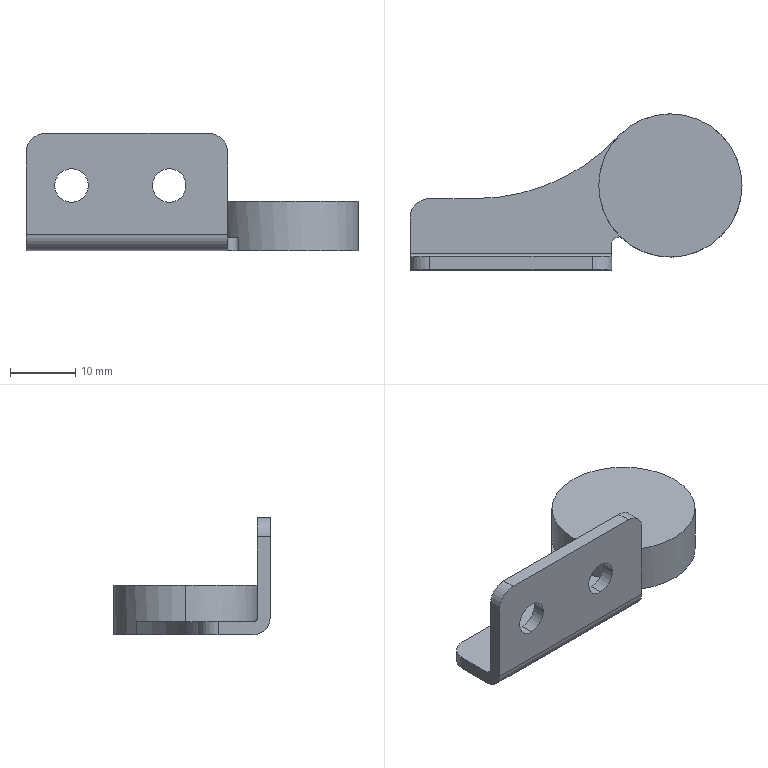Part | SolidWorks | features BaseBody 1 | 1 solid | 42 faces | box 51 x 24 x 18 mm | volume 4464 mm3 | cylinder 25 | plane 17 | commonest cylinder face diameters 0.528 x8 5.153 x4 6 x3 10 x2 10.02 x2 22 x2
STEP:
#1=CARTESIAN_POINT('',(-8.035,10.178,3.237));
#2=VERTEX_POINT('',#1);
#3=CARTESIAN_POINT('',(-11.,2.666,3.237));
#4=VERTEX_POINT('',#3);
#5=CARTESIAN_POINT('',(0.,2.666,3.237));
#6=DIRECTION('',(0.,0.,1.));
#7=DIRECTION('',(1.,0.,0.));
#8=AXIS2_PLACEMENT_3D('',#5,#6,#7);
#9=CIRCLE('',#8,11.);
#10=EDGE_CURVE('',#2,#4,#9,.T.);
#11=ORIENTED_EDGE('',*,*,#10,.T.);
#12=CARTESIAN_POINT('',(-11.,2.666,8.837));
#13=VERTEX_POINT('',#12);
#14=CARTESIAN_POINT('',(-11.,2.666,1.237));
#15=DIRECTION('',(0.,0.,1.));
#16=VECTOR('',#15,1000.);
#17=LINE('',#14,#16);
#18=EDGE_CURVE('',#4,#13,#17,.T.);
#19=ORIENTED_EDGE('',*,*,#18,.T.);
#20=CARTESIAN_POINT('',(11.,2.666,8.837));
#21=VERTEX_POINT('',#20);
#22=CARTESIAN_POINT('',(0.,2.666,8.837));
#23=DIRECTION('',(0.,0.,-1.));
#24=DIRECTION('',(1.,0.,0.));
#25=AXIS2_PLACEMENT_3D('',#22,#23,#24);
#26=CIRCLE('',#25,11.);
#27=EDGE_CURVE('',#13,#21,#26,.T.);
#28=ORIENTED_EDGE('',*,*,#27,.T.);
#29=CARTESIAN_POINT('',(11.,2.666,1.237));
#30=VERTEX_POINT('',#29);
#31=CARTESIAN_POINT('',(11.,2.666,1.237));
#32=DIRECTION('',(0.,0.,1.));
#33=VECTOR('',#32,1000.);
#34=LINE('',#31,#33);
#35=EDGE_CURVE('',#30,#21,#34,.T.);
#36=ORIENTED_EDGE('',*,*,#35,.F.);
#37=CARTESIAN_POINT('',(-8.035,10.178,1.237));
#38=VERTEX_POINT('',#37);
#39=CARTESIAN_POINT('',(0.,2.666,1.237));
#40=DIRECTION('',(0.,0.,-1.));
#41=DIRECTION('',(1.,0.,0.));
#42=AXIS2_PLACEMENT_3D('',#39,#40,#41);
#43=CIRCLE('',#42,11.);
#44=EDGE_CURVE('',#38,#30,#43,.T.);
#45=ORIENTED_EDGE('',*,*,#44,.F.);
#46=CARTESIAN_POINT('',(-8.035,10.178,1.237));
#47=DIRECTION('',(0.,0.,1.));
#48=VECTOR('',#47,1000.);
#49=LINE('',#46,#48);
#50=EDGE_CURVE('',#38,#2,#49,.T.);
#51=ORIENTED_EDGE('',*,*,#50,.T.);
#52=EDGE_LOOP('',(#11,#19,#28,#36,#45,#51));
#53=FACE_OUTER_BOUND('',#52,.T.);
#54=CARTESIAN_POINT('',(0.,2.666,1.237));
#55=DIRECTION('',(0.,0.,1.));
#56=DIRECTION('',(1.,0.,0.));
#57=AXIS2_PLACEMENT_3D('',#54,#55,#56);
#58=CYLINDRICAL_SURFACE('',#57,11.);
#59=ADVANCED_FACE('',(#53),#58,.T.);
#60=CARTESIAN_POINT('',(5.,2.666,1.237));
#61=VERTEX_POINT('',#60);
#62=CARTESIAN_POINT('',(-5.,2.666,1.237));
#63=VERTEX_POINT('',#62);
#64=CARTESIAN_POINT('',(0.,2.666,1.237));
#65=DIRECTION('',(0.,0.,1.));
#66=DIRECTION('',(1.,0.,0.));
#67=AXIS2_PLACEMENT_3D('',#64,#65,#66);
#68=CIRCLE('',#67,5.);
#69=EDGE_CURVE('',#61,#63,#68,.T.);
#70=ORIENTED_EDGE('',*,*,#69,.T.);
#71=CARTESIAN_POINT('',(-5.,2.666,3.237));
#72=VERTEX_POINT('',#71);
#73=CARTESIAN_POINT('',(-5.,2.666,57.799));
#74=DIRECTION('',(0.,0.,1.));
#75=VECTOR('',#74,1000.);
#76=LINE('',#73,#75);
#77=EDGE_CURVE('',#63,#72,#76,.T.);
#78=ORIENTED_EDGE('',*,*,#77,.T.);
#79=CARTESIAN_POINT('',(5.,2.666,3.237));
#80=VERTEX_POINT('',#79);
#81=CARTESIAN_POINT('',(0.,2.666,3.237));
#82=DIRECTION('',(0.,0.,1.));
#83=DIRECTION('',(1.,0.,0.));
#84=AXIS2_PLACEMENT_3D('',#81,#82,#83);
#85=CIRCLE('',#84,5.);
#86=EDGE_CURVE('',#80,#72,#85,.T.);
#87=ORIENTED_EDGE('',*,*,#86,.F.);
#88=CARTESIAN_POINT('',(5.,2.666,57.799));
#89=DIRECTION('',(0.,0.,1.));
#90=VECTOR('',#89,1000.);
#91=LINE('',#88,#90);
#92=EDGE_CURVE('',#61,#80,#91,.T.);
#93=ORIENTED_EDGE('',*,*,#92,.F.);
#94=EDGE_LOOP('',(#70,#78,#87,#93));
#95=FACE_OUTER_BOUND('',#94,.T.);
#96=CARTESIAN_POINT('',(0.,2.666,57.799));
#97=DIRECTION('',(0.,0.,1.));
#98=DIRECTION('',(1.,0.,0.));
#99=AXIS2_PLACEMENT_3D('',#96,#97,#98);
#100=CYLINDRICAL_SURFACE('',#99,5.);
#101=ADVANCED_FACE('',(#95),#100,.T.);
#102=CARTESIAN_POINT('',(-18.,-10.334,13.814));
#103=VERTEX_POINT('',#102);
#104=CARTESIAN_POINT('',(-18.,-10.334,8.66));
#105=VERTEX_POINT('',#104);
#106=CARTESIAN_POINT('',(-18.,-10.334,11.237));
#107=DIRECTION('',(0.,-1.,0.));
#108=DIRECTION('',(0.,0.,1.));
#109=AXIS2_PLACEMENT_3D('',#106,#107,#108);
#110=CIRCLE('',#109,2.577);
#111=EDGE_CURVE('',#103,#105,#110,.T.);
#112=ORIENTED_EDGE('',*,*,#111,.T.);
#113=CARTESIAN_POINT('',(-18.,-8.334,8.66));
#114=VERTEX_POINT('',#113);
#115=CARTESIAN_POINT('',(-18.,-10.334,8.66));
#116=DIRECTION('',(0.,1.,0.));
#117=VECTOR('',#116,1000.);
#118=LINE('',#115,#117);
#119=EDGE_CURVE('',#105,#114,#118,.T.);
#120=ORIENTED_EDGE('',*,*,#119,.T.);
#121=CARTESIAN_POINT('',(-18.,-8.334,13.814));
#122=VERTEX_POINT('',#121);
#123=CARTESIAN_POINT('',(-18.,-8.334,11.237));
#124=DIRECTION('',(0.,-1.,0.));
#125=DIRECTION('',(0.,0.,1.));
#126=AXIS2_PLACEMENT_3D('',#123,#124,#125);
#127=CIRCLE('',#126,2.577);
#128=EDGE_CURVE('',#122,#114,#127,.T.);
#129=ORIENTED_EDGE('',*,*,#128,.F.);
#130=CARTESIAN_POINT('',(-18.,-10.334,13.814));
#131=DIRECTION('',(0.,1.,0.));
#132=VECTOR('',#131,1000.);
#133=LINE('',#130,#132);
#134=EDGE_CURVE('',#103,#122,#133,.T.);
#135=ORIENTED_EDGE('',*,*,#134,.F.);
#136=EDGE_LOOP('',(#112,#120,#129,#135));
#137=FACE_OUTER_BOUND('',#136,.T.);
#138=CARTESIAN_POINT('',(-18.,-10.334,11.237));
#139=DIRECTION('',(0.,1.,0.));
#140=DIRECTION('',(0.,0.,1.));
#141=AXIS2_PLACEMENT_3D('',#138,#139,#140);
#142=CYLINDRICAL_SURFACE('',#141,2.577);
#143=ADVANCED_FACE('',(#137),#142,.F.);
#144=CARTESIAN_POINT('',(-33.,-10.334,13.814));
#145=VERTEX_POINT('',#144);
#146=CARTESIAN_POINT('',(-33.,-10.334,8.66));
#147=VERTEX_POINT('',#146);
#148=CARTESIAN_POINT('',(-33.,-10.334,11.237));
#149=DIRECTION('',(0.,-1.,0.));
#150=DIRECTION('',(0.,0.,1.));
#151=AXIS2_PLACEMENT_3D('',#148,#149,#150);
#152=CIRCLE('',#151,2.577);
#153=EDGE_CURVE('',#145,#147,#152,.T.);
#154=ORIENTED_EDGE('',*,*,#153,.T.);
#155=CARTESIAN_POINT('',(-33.,-8.334,8.66));
#156=VERTEX_POINT('',#155);
#157=CARTESIAN_POINT('',(-33.,-10.334,8.66));
#158=DIRECTION('',(0.,1.,0.));
#159=VECTOR('',#158,1000.);
#160=LINE('',#157,#159);
#161=EDGE_CURVE('',#147,#156,#160,.T.);
#162=ORIENTED_EDGE('',*,*,#161,.T.);
#163=CARTESIAN_POINT('',(-33.,-8.334,13.814));
#164=VERTEX_POINT('',#163);
#165=CARTESIAN_POINT('',(-33.,-8.334,11.237));
#166=DIRECTION('',(0.,-1.,0.));
#167=DIRECTION('',(0.,0.,1.));
#168=AXIS2_PLACEMENT_3D('',#165,#166,#167);
#169=CIRCLE('',#168,2.577);
#170=EDGE_CURVE('',#164,#156,#169,.T.);
#171=ORIENTED_EDGE('',*,*,#170,.F.);
#172=CARTESIAN_POINT('',(-33.,-10.334,13.814));
#173=DIRECTION('',(0.,1.,0.));
#174=VECTOR('',#173,1000.);
#175=LINE('',#172,#174);
#176=EDGE_CURVE('',#145,#164,#175,.T.);
#177=ORIENTED_EDGE('',*,*,#176,.F.);
#178=EDGE_LOOP('',(#154,#162,#171,#177));
#179=FACE_OUTER_BOUND('',#178,.T.);
#180=CARTESIAN_POINT('',(-33.,-10.334,11.237));
#181=DIRECTION('',(0.,1.,0.));
#182=DIRECTION('',(0.,0.,1.));
#183=AXIS2_PLACEMENT_3D('',#180,#181,#182);
#184=CYLINDRICAL_SURFACE('',#183,2.577);
#185=ADVANCED_FACE('',(#179),#184,.F.);
#186=CARTESIAN_POINT('',(4.321,-0.09406,1.237));
#187=VERTEX_POINT('',#186);
#188=CARTESIAN_POINT('',(4.105,-0.2067,1.237));
#189=VERTEX_POINT('',#188);
#190=CARTESIAN_POINT('',(4.321,-0.3581,1.237));
#191=DIRECTION('',(0.,0.,1.));
#192=DIRECTION('',(1.,0.,0.));
#193=AXIS2_PLACEMENT_3D('',#190,#191,#192);
#194=CIRCLE('',#193,0.264);
#195=EDGE_CURVE('',#187,#189,#194,.T.);
#196=ORIENTED_EDGE('',*,*,#195,.F.);
#197=CARTESIAN_POINT('',(6.436,-0.09406,1.237));
#198=VERTEX_POINT('',#197);
#199=CARTESIAN_POINT('',(-8.,-0.09406,1.237));
#200=DIRECTION('',(1.,0.,0.));
#201=VECTOR('',#200,1000.);
#202=LINE('',#199,#201);
#203=EDGE_CURVE('',#187,#198,#202,.T.);
#204=ORIENTED_EDGE('',*,*,#203,.T.);
#205=CARTESIAN_POINT('',(6.7,0.1699,1.237));
#206=VERTEX_POINT('',#205);
#207=CARTESIAN_POINT('',(6.436,0.1699,1.237));
#208=DIRECTION('',(0.,0.,1.));
#209=DIRECTION('',(1.,0.,0.));
#210=AXIS2_PLACEMENT_3D('',#207,#208,#209);
#211=CIRCLE('',#210,0.264);
#212=EDGE_CURVE('',#198,#206,#211,.T.);
#213=ORIENTED_EDGE('',*,*,#212,.T.);
#214=CARTESIAN_POINT('',(6.7,5.162,1.237));
#215=VERTEX_POINT('',#214);
#216=CARTESIAN_POINT('',(6.7,-6.278,1.237));
#217=DIRECTION('',(0.,1.,0.));
#218=VECTOR('',#217,1000.);
#219=LINE('',#216,#218);
#220=EDGE_CURVE('',#206,#215,#219,.T.);
#221=ORIENTED_EDGE('',*,*,#220,.T.);
#222=CARTESIAN_POINT('',(6.436,5.426,1.237));
#223=VERTEX_POINT('',#222);
#224=CARTESIAN_POINT('',(6.436,5.162,1.237));
#225=DIRECTION('',(0.,0.,1.));
#226=DIRECTION('',(1.,0.,0.));
#227=AXIS2_PLACEMENT_3D('',#224,#225,#226);
#228=CIRCLE('',#227,0.264);
#229=EDGE_CURVE('',#215,#223,#228,.T.);
#230=ORIENTED_EDGE('',*,*,#229,.T.);
#231=CARTESIAN_POINT('',(4.321,5.426,1.237));
#232=VERTEX_POINT('',#231);
#233=CARTESIAN_POINT('',(-8.,5.426,1.237));
#234=DIRECTION('',(-1.,0.,0.));
#235=VECTOR('',#234,1000.);
#236=LINE('',#233,#235);
#237=EDGE_CURVE('',#223,#232,#236,.T.);
#238=ORIENTED_EDGE('',*,*,#237,.T.);
#239=CARTESIAN_POINT('',(4.105,5.539,1.237));
#240=VERTEX_POINT('',#239);
#241=CARTESIAN_POINT('',(4.321,5.69,1.237));
#242=DIRECTION('',(0.,0.,1.));
#243=DIRECTION('',(1.,0.,0.));
#244=AXIS2_PLACEMENT_3D('',#241,#242,#243);
#245=CIRCLE('',#244,0.264);
#246=EDGE_CURVE('',#240,#232,#245,.T.);
#247=ORIENTED_EDGE('',*,*,#246,.F.);
#248=CARTESIAN_POINT('',(-4.105,5.539,1.237));
#249=VERTEX_POINT('',#248);
#250=CARTESIAN_POINT('',(0.,2.666,1.237));
#251=DIRECTION('',(0.,0.,1.));
#252=DIRECTION('',(1.,0.,0.));
#253=AXIS2_PLACEMENT_3D('',#250,#251,#252);
#254=CIRCLE('',#253,5.01);
#255=EDGE_CURVE('',#240,#249,#254,.T.);
#256=ORIENTED_EDGE('',*,*,#255,.T.);
#257=CARTESIAN_POINT('',(-4.321,5.426,1.237));
#258=VERTEX_POINT('',#257);
#259=CARTESIAN_POINT('',(-4.321,5.69,1.237));
#260=DIRECTION('',(0.,0.,1.));
#261=DIRECTION('',(1.,0.,0.));
#262=AXIS2_PLACEMENT_3D('',#259,#260,#261);
#263=CIRCLE('',#262,0.264);
#264=EDGE_CURVE('',#258,#249,#263,.T.);
#265=ORIENTED_EDGE('',*,*,#264,.F.);
#266=CARTESIAN_POINT('',(-6.436,5.426,1.237));
#267=VERTEX_POINT('',#266);
#268=CARTESIAN_POINT('',(-8.,5.426,1.237));
#269=DIRECTION('',(-1.,0.,0.));
#270=VECTOR('',#269,1000.);
#271=LINE('',#268,#270);
#272=EDGE_CURVE('',#258,#267,#271,.T.);
#273=ORIENTED_EDGE('',*,*,#272,.T.);
#274=CARTESIAN_POINT('',(-6.7,5.162,1.237));
#275=VERTEX_POINT('',#274);
#276=CARTESIAN_POINT('',(-6.436,5.162,1.237));
#277=DIRECTION('',(0.,0.,1.));
#278=DIRECTION('',(1.,0.,0.));
#279=AXIS2_PLACEMENT_3D('',#276,#277,#278);
#280=CIRCLE('',#279,0.264);
#281=EDGE_CURVE('',#267,#275,#280,.T.);
#282=ORIENTED_EDGE('',*,*,#281,.T.);
#283=CARTESIAN_POINT('',(-6.7,0.1699,1.237));
#284=VERTEX_POINT('',#283);
#285=CARTESIAN_POINT('',(-6.7,-6.278,1.237));
#286=DIRECTION('',(0.,-1.,0.));
#287=VECTOR('',#286,1000.);
#288=LINE('',#285,#287);
#289=EDGE_CURVE('',#275,#284,#288,.T.);
#290=ORIENTED_EDGE('',*,*,#289,.T.);
#291=CARTESIAN_POINT('',(-6.436,-0.09406,1.237));
#292=VERTEX_POINT('',#291);
#293=CARTESIAN_POINT('',(-6.436,0.1699,1.237));
#294=DIRECTION('',(0.,0.,1.));
#295=DIRECTION('',(1.,0.,0.));
#296=AXIS2_PLACEMENT_3D('',#293,#294,#295);
#297=CIRCLE('',#296,0.264);
#298=EDGE_CURVE('',#284,#292,#297,.T.);
#299=ORIENTED_EDGE('',*,*,#298,.T.);
#300=CARTESIAN_POINT('',(-4.321,-0.09406,1.237));
#301=VERTEX_POINT('',#300);
#302=CARTESIAN_POINT('',(-8.,-0.09406,1.237));
#303=DIRECTION('',(1.,0.,0.));
#304=VECTOR('',#303,1000.);
#305=LINE('',#302,#304);
#306=EDGE_CURVE('',#292,#301,#305,.T.);
#307=ORIENTED_EDGE('',*,*,#306,.T.);
#308=CARTESIAN_POINT('',(-4.105,-0.2067,1.237));
#309=VERTEX_POINT('',#308);
#310=CARTESIAN_POINT('',(-4.321,-0.3581,1.237));
#311=DIRECTION('',(0.,0.,1.));
#312=DIRECTION('',(1.,0.,0.));
#313=AXIS2_PLACEMENT_3D('',#310,#311,#312);
#314=CIRCLE('',#313,0.264);
#315=EDGE_CURVE('',#309,#301,#314,.T.);
#316=ORIENTED_EDGE('',*,*,#315,.F.);
#317=CARTESIAN_POINT('',(0.,2.666,1.237));
#318=DIRECTION('',(0.,0.,1.));
#319=DIRECTION('',(1.,0.,0.));
#320=AXIS2_PLACEMENT_3D('',#317,#318,#319);
#321=CIRCLE('',#320,5.01);
#322=EDGE_CURVE('',#309,#189,#321,.T.);
#323=ORIENTED_EDGE('',*,*,#322,.T.);
#324=EDGE_LOOP('',(#196,#204,#213,#221,#230,#238,#247,#256,#265,#273,#282,#290,#299,#307,#316,#323));
#325=FACE_BOUND('',#324,.T.);
#326=ORIENTED_EDGE('',*,*,#44,.T.);
#327=CARTESIAN_POINT('',(-7.333,-5.533,1.237));
#328=VERTEX_POINT('',#327);
#329=CARTESIAN_POINT('',(0.,2.666,1.237));
#330=DIRECTION('',(0.,0.,-1.));
#331=DIRECTION('',(1.,0.,0.));
#332=AXIS2_PLACEMENT_3D('',#329,#330,#331);
#333=CIRCLE('',#332,11.);
#334=EDGE_CURVE('',#30,#328,#333,.T.);
#335=ORIENTED_EDGE('',*,*,#334,.T.);
#336=CARTESIAN_POINT('',(-9.,-6.278,1.237));
#337=VERTEX_POINT('',#336);
#338=CARTESIAN_POINT('',(-8.,-6.278,1.237));
#339=DIRECTION('',(0.,0.,1.));
#340=DIRECTION('',(1.,0.,0.));
#341=AXIS2_PLACEMENT_3D('',#338,#339,#340);
#342=CIRCLE('',#341,1.);
#343=EDGE_CURVE('',#328,#337,#342,.T.);
#344=ORIENTED_EDGE('',*,*,#343,.T.);
#345=CARTESIAN_POINT('',(-9.,-7.834,1.237));
#346=VERTEX_POINT('',#345);
#347=CARTESIAN_POINT('',(-9.,-10.334,1.237));
#348=DIRECTION('',(0.,1.,0.));
#349=VECTOR('',#348,1000.);
#350=LINE('',#347,#349);
#351=EDGE_CURVE('',#346,#337,#350,.T.);
#352=ORIENTED_EDGE('',*,*,#351,.F.);
#353=CARTESIAN_POINT('',(-40.,-7.834,1.237));
#354=VERTEX_POINT('',#353);
#355=CARTESIAN_POINT('',(-8.,-7.834,1.237));
#356=DIRECTION('',(-1.,0.,0.));
#357=VECTOR('',#356,1000.);
#358=LINE('',#355,#357);
#359=EDGE_CURVE('',#346,#354,#358,.T.);
#360=ORIENTED_EDGE('',*,*,#359,.T.);
#361=CARTESIAN_POINT('',(-40.,-2.334,1.237));
#362=VERTEX_POINT('',#361);
#363=CARTESIAN_POINT('',(-40.,-6.278,1.237));
#364=DIRECTION('',(0.,1.,0.));
#365=VECTOR('',#364,1000.);
#366=LINE('',#363,#365);
#367=EDGE_CURVE('',#354,#362,#366,.T.);
#368=ORIENTED_EDGE('',*,*,#367,.T.);
#369=CARTESIAN_POINT('',(-37.,0.6659,1.237));
#370=VERTEX_POINT('',#369);
#371=CARTESIAN_POINT('',(-37.,-2.334,1.237));
#372=DIRECTION('',(0.,0.,-1.));
#373=DIRECTION('',(1.,0.,0.));
#374=AXIS2_PLACEMENT_3D('',#371,#372,#373);
#375=CIRCLE('',#374,3.);
#376=EDGE_CURVE('',#362,#370,#375,.T.);
#377=ORIENTED_EDGE('',*,*,#376,.T.);
#378=CARTESIAN_POINT('',(-29.95,0.6659,1.237));
#379=VERTEX_POINT('',#378);
#380=CARTESIAN_POINT('',(-8.,0.6659,1.237));
#381=DIRECTION('',(1.,0.,0.));
#382=VECTOR('',#381,1000.);
#383=LINE('',#380,#382);
#384=EDGE_CURVE('',#370,#379,#383,.T.);
#385=ORIENTED_EDGE('',*,*,#384,.T.);
#386=CARTESIAN_POINT('',(-29.95,30.666,1.237));
#387=DIRECTION('',(0.,0.,1.));
#388=DIRECTION('',(1.,0.,0.));
#389=AXIS2_PLACEMENT_3D('',#386,#387,#388);
#390=CIRCLE('',#389,30.);
#391=EDGE_CURVE('',#379,#38,#390,.T.);
#392=ORIENTED_EDGE('',*,*,#391,.T.);
#393=EDGE_LOOP('',(#326,#335,#344,#352,#360,#368,#377,#385,#392));
#394=FACE_OUTER_BOUND('',#393,.T.);
#395=CARTESIAN_POINT('',(-8.,-6.278,1.237));
#396=DIRECTION('',(0.,0.,-1.));
#397=DIRECTION('',(-1.,0.,0.));
#398=AXIS2_PLACEMENT_3D('',#395,#396,#397);
#399=PLANE('',#398);
#400=ADVANCED_FACE('',(#325,#394),#399,.T.);
#401=CARTESIAN_POINT('',(6.436,-0.09406,3.237));
#402=VERTEX_POINT('',#401);
#403=CARTESIAN_POINT('',(6.436,-0.09406,1.237));
#404=DIRECTION('',(0.,0.,1.));
#405=VECTOR('',#404,1000.);
#406=LINE('',#403,#405);
#407=EDGE_CURVE('',#198,#402,#406,.T.);
#408=ORIENTED_EDGE('',*,*,#407,.F.);
#409=ORIENTED_EDGE('',*,*,#203,.F.);
#410=CARTESIAN_POINT('',(4.321,-0.09406,3.237));
#411=VERTEX_POINT('',#410);
#412=CARTESIAN_POINT('',(4.321,-0.09406,1.237));
#413=DIRECTION('',(0.,0.,-1.));
#414=VECTOR('',#413,1000.);
#415=LINE('',#412,#414);
#416=EDGE_CURVE('',#411,#187,#415,.T.);
#417=ORIENTED_EDGE('',*,*,#416,.F.);
#418=CARTESIAN_POINT('',(4.321,-0.09406,3.237));
#419=DIRECTION('',(-1.,0.,0.));
#420=VECTOR('',#419,1000.);
#421=LINE('',#418,#420);
#422=EDGE_CURVE('',#402,#411,#421,.T.);
#423=ORIENTED_EDGE('',*,*,#422,.F.);
#424=EDGE_LOOP('',(#408,#409,#417,#423));
#425=FACE_OUTER_BOUND('',#424,.T.);
#426=CARTESIAN_POINT('',(4.321,-0.09406,1.237));
#427=DIRECTION('',(0.,-1.,0.));
#428=DIRECTION('',(0.,0.,-1.));
#429=AXIS2_PLACEMENT_3D('',#426,#427,#428);
#430=PLANE('',#429);
#431=ADVANCED_FACE('',(#425),#430,.F.);
#432=CARTESIAN_POINT('',(4.105,-0.2067,3.237));
#433=VERTEX_POINT('',#432);
#434=CARTESIAN_POINT('',(4.105,-0.2067,1.237));
#435=DIRECTION('',(0.,0.,1.));
#436=VECTOR('',#435,1000.);
#437=LINE('',#434,#436);
#438=EDGE_CURVE('',#189,#433,#437,.T.);
#439=ORIENTED_EDGE('',*,*,#438,.F.);
#440=ORIENTED_EDGE('',*,*,#322,.F.);
#441=CARTESIAN_POINT('',(-4.105,-0.2067,3.237));
#442=VERTEX_POINT('',#441);
#443=CARTESIAN_POINT('',(-4.105,-0.2067,1.237));
#444=DIRECTION('',(0.,0.,-1.));
#445=VECTOR('',#444,1000.);
#446=LINE('',#443,#445);
#447=EDGE_CURVE('',#442,#309,#446,.T.);
#448=ORIENTED_EDGE('',*,*,#447,.F.);
#449=CARTESIAN_POINT('',(0.,2.666,3.237));
#450=DIRECTION('',(0.,0.,-1.));
#451=DIRECTION('',(1.,0.,0.));
#452=AXIS2_PLACEMENT_3D('',#449,#450,#451);
#453=CIRCLE('',#452,5.01);
#454=EDGE_CURVE('',#433,#442,#453,.T.);
#455=ORIENTED_EDGE('',*,*,#454,.F.);
#456=EDGE_LOOP('',(#439,#440,#448,#455));
#457=FACE_OUTER_BOUND('',#456,.T.);
#458=CARTESIAN_POINT('',(0.,2.666,1.237));
#459=DIRECTION('',(0.,0.,1.));
#460=DIRECTION('',(1.,0.,0.));
#461=AXIS2_PLACEMENT_3D('',#458,#459,#460);
#462=CYLINDRICAL_SURFACE('',#461,5.01);
#463=ADVANCED_FACE('',(#457),#462,.F.);
#464=CARTESIAN_POINT('',(-4.321,-0.09406,3.237));
#465=VERTEX_POINT('',#464);
#466=CARTESIAN_POINT('',(-4.321,-0.09406,1.237));
#467=DIRECTION('',(0.,0.,1.));
#468=VECTOR('',#467,1000.);
#469=LINE('',#466,#468);
#470=EDGE_CURVE('',#301,#465,#469,.T.);
#471=ORIENTED_EDGE('',*,*,#470,.F.);
#472=ORIENTED_EDGE('',*,*,#306,.F.);
#473=CARTESIAN_POINT('',(-6.436,-0.09406,3.237));
#474=VERTEX_POINT('',#473);
#475=CARTESIAN_POINT('',(-6.436,-0.09406,1.237));
#476=DIRECTION('',(0.,0.,-1.));
#477=VECTOR('',#476,1000.);
#478=LINE('',#475,#477);
#479=EDGE_CURVE('',#474,#292,#478,.T.);
#480=ORIENTED_EDGE('',*,*,#479,.F.);
#481=CARTESIAN_POINT('',(-6.436,-0.09406,3.237));
#482=DIRECTION('',(-1.,0.,0.));
#483=VECTOR('',#482,1000.);
#484=LINE('',#481,#483);
#485=EDGE_CURVE('',#465,#474,#484,.T.);
#486=ORIENTED_EDGE('',*,*,#485,.F.);
#487=EDGE_LOOP('',(#471,#472,#480,#486));
#488=FACE_OUTER_BOUND('',#487,.T.);
#489=CARTESIAN_POINT('',(-6.436,-0.09406,1.237));
#490=DIRECTION('',(0.,-1.,0.));
#491=DIRECTION('',(0.,0.,-1.));
#492=AXIS2_PLACEMENT_3D('',#489,#490,#491);
#493=PLANE('',#492);
#494=ADVANCED_FACE('',(#488),#493,.F.);
#495=CARTESIAN_POINT('',(-6.7,0.1699,3.237));
#496=VERTEX_POINT('',#495);
#497=CARTESIAN_POINT('',(-6.7,0.1699,1.237));
#498=DIRECTION('',(0.,0.,1.));
#499=VECTOR('',#498,1000.);
#500=LINE('',#497,#499);
#501=EDGE_CURVE('',#284,#496,#500,.T.);
#502=ORIENTED_EDGE('',*,*,#501,.F.);
#503=ORIENTED_EDGE('',*,*,#289,.F.);
#504=CARTESIAN_POINT('',(-6.7,5.162,3.237));
#505=VERTEX_POINT('',#504);
#506=CARTESIAN_POINT('',(-6.7,5.162,1.237));
#507=DIRECTION('',(0.,0.,-1.));
#508=VECTOR('',#507,1000.);
#509=LINE('',#506,#508);
#510=EDGE_CURVE('',#505,#275,#509,.T.);
#511=ORIENTED_EDGE('',*,*,#510,.F.);
#512=CARTESIAN_POINT('',(-6.7,5.162,3.237));
#513=DIRECTION('',(0.,1.,0.));
#514=VECTOR('',#513,1000.);
#515=LINE('',#512,#514);
#516=EDGE_CURVE('',#496,#505,#515,.T.);
#517=ORIENTED_EDGE('',*,*,#516,.F.);
#518=EDGE_LOOP('',(#502,#503,#511,#517));
#519=FACE_OUTER_BOUND('',#518,.T.);
#520=CARTESIAN_POINT('',(-6.7,5.162,1.237));
#521=DIRECTION('',(-1.,0.,0.));
#522=DIRECTION('',(0.,-1.,0.));
#523=AXIS2_PLACEMENT_3D('',#520,#521,#522);
#524=PLANE('',#523);
#525=ADVANCED_FACE('',(#519),#524,.F.);
#526=CARTESIAN_POINT('',(-6.436,5.426,3.237));
#527=VERTEX_POINT('',#526);
#528=CARTESIAN_POINT('',(-6.436,5.426,1.237));
#529=DIRECTION('',(0.,0.,1.));
#530=VECTOR('',#529,1000.);
#531=LINE('',#528,#530);
#532=EDGE_CURVE('',#267,#527,#531,.T.);
#533=ORIENTED_EDGE('',*,*,#532,.F.);
#534=ORIENTED_EDGE('',*,*,#272,.F.);
#535=CARTESIAN_POINT('',(-4.321,5.426,3.237));
#536=VERTEX_POINT('',#535);
#537=CARTESIAN_POINT('',(-4.321,5.426,1.237));
#538=DIRECTION('',(0.,0.,-1.));
#539=VECTOR('',#538,1000.);
#540=LINE('',#537,#539);
#541=EDGE_CURVE('',#536,#258,#540,.T.);
#542=ORIENTED_EDGE('',*,*,#541,.F.);
#543=CARTESIAN_POINT('',(-6.436,5.426,3.237));
#544=DIRECTION('',(1.,0.,0.));
#545=VECTOR('',#544,1000.);
#546=LINE('',#543,#545);
#547=EDGE_CURVE('',#527,#536,#546,.T.);
#548=ORIENTED_EDGE('',*,*,#547,.F.);
#549=EDGE_LOOP('',(#533,#534,#542,#548));
#550=FACE_OUTER_BOUND('',#549,.T.);
#551=CARTESIAN_POINT('',(-6.436,5.426,1.237));
#552=DIRECTION('',(0.,1.,0.));
#553=DIRECTION('',(0.,0.,1.));
#554=AXIS2_PLACEMENT_3D('',#551,#552,#553);
#555=PLANE('',#554);
#556=ADVANCED_FACE('',(#550),#555,.F.);
#557=CARTESIAN_POINT('',(-4.105,5.539,3.237));
#558=VERTEX_POINT('',#557);
#559=CARTESIAN_POINT('',(-4.105,5.539,1.237));
#560=DIRECTION('',(0.,0.,1.));
#561=VECTOR('',#560,1000.);
#562=LINE('',#559,#561);
#563=EDGE_CURVE('',#249,#558,#562,.T.);
#564=ORIENTED_EDGE('',*,*,#563,.F.);
#565=ORIENTED_EDGE('',*,*,#255,.F.);
#566=CARTESIAN_POINT('',(4.105,5.539,3.237));
#567=VERTEX_POINT('',#566);
#568=CARTESIAN_POINT('',(4.105,5.539,1.237));
#569=DIRECTION('',(0.,0.,-1.));
#570=VECTOR('',#569,1000.);
#571=LINE('',#568,#570);
#572=EDGE_CURVE('',#567,#240,#571,.T.);
#573=ORIENTED_EDGE('',*,*,#572,.F.);
#574=CARTESIAN_POINT('',(0.,2.666,3.237));
#575=DIRECTION('',(0.,0.,-1.));
#576=DIRECTION('',(1.,0.,0.));
#577=AXIS2_PLACEMENT_3D('',#574,#575,#576);
#578=CIRCLE('',#577,5.01);
#579=EDGE_CURVE('',#558,#567,#578,.T.);
#580=ORIENTED_EDGE('',*,*,#579,.F.);
#581=EDGE_LOOP('',(#564,#565,#573,#580));
#582=FACE_OUTER_BOUND('',#581,.T.);
#583=CARTESIAN_POINT('',(0.,2.666,1.237));
#584=DIRECTION('',(0.,0.,1.));
#585=DIRECTION('',(1.,0.,0.));
#586=AXIS2_PLACEMENT_3D('',#583,#584,#585);
#587=CYLINDRICAL_SURFACE('',#586,5.01);
#588=ADVANCED_FACE('',(#582),#587,.F.);
#589=CARTESIAN_POINT('',(4.321,5.426,3.237));
#590=VERTEX_POINT('',#589);
#591=CARTESIAN_POINT('',(4.321,5.426,1.237));
#592=DIRECTION('',(0.,0.,1.));
#593=VECTOR('',#592,1000.);
#594=LINE('',#591,#593);
#595=EDGE_CURVE('',#232,#590,#594,.T.);
#596=ORIENTED_EDGE('',*,*,#595,.F.);
#597=ORIENTED_EDGE('',*,*,#237,.F.);
#598=CARTESIAN_POINT('',(6.436,5.426,3.237));
#599=VERTEX_POINT('',#598);
#600=CARTESIAN_POINT('',(6.436,5.426,1.237));
#601=DIRECTION('',(0.,0.,-1.));
#602=VECTOR('',#601,1000.);
#603=LINE('',#600,#602);
#604=EDGE_CURVE('',#599,#223,#603,.T.);
#605=ORIENTED_EDGE('',*,*,#604,.F.);
#606=CARTESIAN_POINT('',(4.321,5.426,3.237));
#607=DIRECTION('',(1.,0.,0.));
#608=VECTOR('',#607,1000.);
#609=LINE('',#606,#608);
#610=EDGE_CURVE('',#590,#599,#609,.T.);
#611=ORIENTED_EDGE('',*,*,#610,.F.);
#612=EDGE_LOOP('',(#596,#597,#605,#611));
#613=FACE_OUTER_BOUND('',#612,.T.);
#614=CARTESIAN_POINT('',(4.321,5.426,1.237));
#615=DIRECTION('',(0.,1.,0.));
#616=DIRECTION('',(0.,0.,1.));
#617=AXIS2_PLACEMENT_3D('',#614,#615,#616);
#618=PLANE('',#617);
#619=ADVANCED_FACE('',(#613),#618,.F.);
#620=CARTESIAN_POINT('',(6.7,5.162,3.237));
#621=VERTEX_POINT('',#620);
#622=CARTESIAN_POINT('',(6.7,5.162,1.237));
#623=DIRECTION('',(0.,0.,1.));
#624=VECTOR('',#623,1000.);
#625=LINE('',#622,#624);
#626=EDGE_CURVE('',#215,#621,#625,.T.);
#627=ORIENTED_EDGE('',*,*,#626,.F.);
#628=ORIENTED_EDGE('',*,*,#220,.F.);
#629=CARTESIAN_POINT('',(6.7,0.1699,3.237));
#630=VERTEX_POINT('',#629);
#631=CARTESIAN_POINT('',(6.7,0.1699,1.237));
#632=DIRECTION('',(0.,0.,-1.));
#633=VECTOR('',#632,1000.);
#634=LINE('',#631,#633);
#635=EDGE_CURVE('',#630,#206,#634,.T.);
#636=ORIENTED_EDGE('',*,*,#635,.F.);
#637=CARTESIAN_POINT('',(6.7,5.162,3.237));
#638=DIRECTION('',(0.,-1.,0.));
#639=VECTOR('',#638,1000.);
#640=LINE('',#637,#639);
#641=EDGE_CURVE('',#621,#630,#640,.T.);
#642=ORIENTED_EDGE('',*,*,#641,.F.);
#643=EDGE_LOOP('',(#627,#628,#636,#642));
#644=FACE_OUTER_BOUND('',#643,.T.);
#645=CARTESIAN_POINT('',(6.7,5.162,1.237));
#646=DIRECTION('',(1.,0.,0.));
#647=DIRECTION('',(0.,0.,-1.));
#648=AXIS2_PLACEMENT_3D('',#645,#646,#647);
#649=PLANE('',#648);
#650=ADVANCED_FACE('',(#644),#649,.F.);
#651=CARTESIAN_POINT('',(-9.,-6.278,3.237));
#652=VERTEX_POINT('',#651);
#653=CARTESIAN_POINT('',(-9.,-6.278,1.237));
#654=DIRECTION('',(0.,0.,1.));
#655=VECTOR('',#654,1000.);
#656=LINE('',#653,#655);
#657=EDGE_CURVE('',#337,#652,#656,.T.);
#658=ORIENTED_EDGE('',*,*,#657,.F.);
#659=ORIENTED_EDGE('',*,*,#343,.F.);
#660=CARTESIAN_POINT('',(-7.333,-5.533,3.237));
#661=VERTEX_POINT('',#660);
#662=CARTESIAN_POINT('',(-7.333,-5.533,1.237));
#663=DIRECTION('',(0.,0.,-1.));
#664=VECTOR('',#663,1000.);
#665=LINE('',#662,#664);
#666=EDGE_CURVE('',#661,#328,#665,.T.);
#667=ORIENTED_EDGE('',*,*,#666,.F.);
#668=CARTESIAN_POINT('',(-8.,-6.278,3.237));
#669=DIRECTION('',(0.,0.,-1.));
#670=DIRECTION('',(1.,0.,0.));
#671=AXIS2_PLACEMENT_3D('',#668,#669,#670);
#672=CIRCLE('',#671,1.);
#673=EDGE_CURVE('',#652,#661,#672,.T.);
#674=ORIENTED_EDGE('',*,*,#673,.F.);
#675=EDGE_LOOP('',(#658,#659,#667,#674));
#676=FACE_OUTER_BOUND('',#675,.T.);
#677=CARTESIAN_POINT('',(-8.,-6.278,1.237));
#678=DIRECTION('',(0.,0.,1.));
#679=DIRECTION('',(1.,0.,0.));
#680=AXIS2_PLACEMENT_3D('',#677,#678,#679);
#681=CYLINDRICAL_SURFACE('',#680,1.);
#682=ADVANCED_FACE('',(#676),#681,.F.);
#683=ORIENTED_EDGE('',*,*,#18,.F.);
#684=CARTESIAN_POINT('',(0.,2.666,3.237));
#685=DIRECTION('',(0.,0.,1.));
#686=DIRECTION('',(1.,0.,0.));
#687=AXIS2_PLACEMENT_3D('',#684,#685,#686);
#688=CIRCLE('',#687,11.);
#689=EDGE_CURVE('',#4,#661,#688,.T.);
#690=ORIENTED_EDGE('',*,*,#689,.T.);
#691=ORIENTED_EDGE('',*,*,#666,.T.);
#692=ORIENTED_EDGE('',*,*,#334,.F.);
#693=ORIENTED_EDGE('',*,*,#35,.T.);
#694=CARTESIAN_POINT('',(0.,2.666,8.837));
#695=DIRECTION('',(0.,0.,-1.));
#696=DIRECTION('',(1.,0.,0.));
#697=AXIS2_PLACEMENT_3D('',#694,#695,#696);
#698=CIRCLE('',#697,11.);
#699=EDGE_CURVE('',#21,#13,#698,.T.);
#700=ORIENTED_EDGE('',*,*,#699,.T.);
#701=EDGE_LOOP('',(#683,#690,#691,#692,#693,#700));
#702=FACE_OUTER_BOUND('',#701,.T.);
#703=CARTESIAN_POINT('',(0.,2.666,1.237));
#704=DIRECTION('',(0.,0.,1.));
#705=DIRECTION('',(1.,0.,0.));
#706=AXIS2_PLACEMENT_3D('',#703,#704,#705);
#707=CYLINDRICAL_SURFACE('',#706,11.);
#708=ADVANCED_FACE('',(#702),#707,.T.);
#709=ORIENTED_EDGE('',*,*,#50,.F.);
#710=ORIENTED_EDGE('',*,*,#391,.F.);
#711=CARTESIAN_POINT('',(-29.95,0.6659,3.237));
#712=VERTEX_POINT('',#711);
#713=CARTESIAN_POINT('',(-29.95,0.6659,1.237));
#714=DIRECTION('',(0.,0.,-1.));
#715=VECTOR('',#714,1000.);
#716=LINE('',#713,#715);
#717=EDGE_CURVE('',#712,#379,#716,.T.);
#718=ORIENTED_EDGE('',*,*,#717,.F.);
#719=CARTESIAN_POINT('',(-29.95,30.666,3.237));
#720=DIRECTION('',(0.,0.,-1.));
#721=DIRECTION('',(1.,0.,0.));
#722=AXIS2_PLACEMENT_3D('',#719,#720,#721);
#723=CIRCLE('',#722,30.);
#724=EDGE_CURVE('',#2,#712,#723,.T.);
#725=ORIENTED_EDGE('',*,*,#724,.F.);
#726=EDGE_LOOP('',(#709,#710,#718,#725));
#727=FACE_OUTER_BOUND('',#726,.T.);
#728=CARTESIAN_POINT('',(-29.95,30.666,1.237));
#729=DIRECTION('',(0.,0.,1.));
#730=DIRECTION('',(1.,0.,0.));
#731=AXIS2_PLACEMENT_3D('',#728,#729,#730);
#732=CYLINDRICAL_SURFACE('',#731,30.);
#733=ADVANCED_FACE('',(#727),#732,.F.);
#734=ORIENTED_EDGE('',*,*,#384,.F.);
#735=CARTESIAN_POINT('',(-37.,0.6659,3.237));
#736=VERTEX_POINT('',#735);
#737=CARTESIAN_POINT('',(-37.,0.6659,1.237));
#738=DIRECTION('',(0.,0.,1.));
#739=VECTOR('',#738,1000.);
#740=LINE('',#737,#739);
#741=EDGE_CURVE('',#370,#736,#740,.T.);
#742=ORIENTED_EDGE('',*,*,#741,.T.);
#743=CARTESIAN_POINT('',(-29.95,0.6659,3.237));
#744=DIRECTION('',(1.,0.,0.));
#745=VECTOR('',#744,1000.);
#746=LINE('',#743,#745);
#747=EDGE_CURVE('',#736,#712,#746,.T.);
#748=ORIENTED_EDGE('',*,*,#747,.T.);
#749=ORIENTED_EDGE('',*,*,#717,.T.);
#750=EDGE_LOOP('',(#734,#742,#748,#749));
#751=FACE_OUTER_BOUND('',#750,.T.);
#752=CARTESIAN_POINT('',(-29.95,0.6659,1.237));
#753=DIRECTION('',(0.,1.,0.));
#754=DIRECTION('',(0.,0.,1.));
#755=AXIS2_PLACEMENT_3D('',#752,#753,#754);
#756=PLANE('',#755);
#757=ADVANCED_FACE('',(#751),#756,.T.);
#758=ORIENTED_EDGE('',*,*,#376,.F.);
#759=CARTESIAN_POINT('',(-40.,-2.334,3.237));
#760=VERTEX_POINT('',#759);
#761=CARTESIAN_POINT('',(-40.,-2.334,1.237));
#762=DIRECTION('',(0.,0.,1.));
#763=VECTOR('',#762,1000.);
#764=LINE('',#761,#763);
#765=EDGE_CURVE('',#362,#760,#764,.T.);
#766=ORIENTED_EDGE('',*,*,#765,.T.);
#767=CARTESIAN_POINT('',(-37.,-2.334,3.237));
#768=DIRECTION('',(0.,0.,-1.));
#769=DIRECTION('',(1.,0.,0.));
#770=AXIS2_PLACEMENT_3D('',#767,#768,#769);
#771=CIRCLE('',#770,3.);
#772=EDGE_CURVE('',#760,#736,#771,.T.);
#773=ORIENTED_EDGE('',*,*,#772,.T.);
#774=ORIENTED_EDGE('',*,*,#741,.F.);
#775=EDGE_LOOP('',(#758,#766,#773,#774));
#776=FACE_OUTER_BOUND('',#775,.T.);
#777=CARTESIAN_POINT('',(-37.,-2.334,1.237));
#778=DIRECTION('',(0.,0.,1.));
#779=DIRECTION('',(1.,0.,0.));
#780=AXIS2_PLACEMENT_3D('',#777,#778,#779);
#781=CYLINDRICAL_SURFACE('',#780,3.);
#782=ADVANCED_FACE('',(#776),#781,.T.);
#783=ORIENTED_EDGE('',*,*,#765,.F.);
#784=ORIENTED_EDGE('',*,*,#367,.F.);
#785=CARTESIAN_POINT('',(-40.,-10.334,3.737));
#786=VERTEX_POINT('',#785);
#787=CARTESIAN_POINT('',(-40.,-7.834,3.737));
#788=DIRECTION('',(1.,0.,0.));
#789=DIRECTION('',(0.,0.,-1.));
#790=AXIS2_PLACEMENT_3D('',#787,#788,#789);
#791=CIRCLE('',#790,2.5);
#792=EDGE_CURVE('',#786,#354,#791,.T.);
#793=ORIENTED_EDGE('',*,*,#792,.F.);
#794=CARTESIAN_POINT('',(-40.,-10.334,16.237));
#795=VERTEX_POINT('',#794);
#796=CARTESIAN_POINT('',(-40.,-10.334,16.237));
#797=DIRECTION('',(0.,0.,1.));
#798=VECTOR('',#797,1000.);
#799=LINE('',#796,#798);
#800=EDGE_CURVE('',#786,#795,#799,.T.);
#801=ORIENTED_EDGE('',*,*,#800,.T.);
#802=CARTESIAN_POINT('',(-40.,-8.334,16.237));
#803=VERTEX_POINT('',#802);
#804=CARTESIAN_POINT('',(-40.,-10.334,16.237));
#805=DIRECTION('',(0.,-1.,0.));
#806=VECTOR('',#805,1000.);
#807=LINE('',#804,#806);
#808=EDGE_CURVE('',#803,#795,#807,.T.);
#809=ORIENTED_EDGE('',*,*,#808,.F.);
#810=CARTESIAN_POINT('',(-40.,-8.334,3.737));
#811=VERTEX_POINT('',#810);
#812=CARTESIAN_POINT('',(-40.,-8.334,3.237));
#813=DIRECTION('',(0.,0.,1.));
#814=VECTOR('',#813,1000.);
#815=LINE('',#812,#814);
#816=EDGE_CURVE('',#811,#803,#815,.T.);
#817=ORIENTED_EDGE('',*,*,#816,.F.);
#818=CARTESIAN_POINT('',(-40.,-7.834,3.237));
#819=VERTEX_POINT('',#818);
#820=CARTESIAN_POINT('',(-40.,-7.834,3.737));
#821=DIRECTION('',(1.,0.,0.));
#822=DIRECTION('',(0.,0.,-1.));
#823=AXIS2_PLACEMENT_3D('',#820,#821,#822);
#824=CIRCLE('',#823,0.5);
#825=EDGE_CURVE('',#811,#819,#824,.T.);
#826=ORIENTED_EDGE('',*,*,#825,.T.);
#827=CARTESIAN_POINT('',(-40.,-2.334,3.237));
#828=DIRECTION('',(0.,1.,0.));
#829=VECTOR('',#828,1000.);
#830=LINE('',#827,#829);
#831=EDGE_CURVE('',#819,#760,#830,.T.);
#832=ORIENTED_EDGE('',*,*,#831,.T.);
#833=EDGE_LOOP('',(#783,#784,#793,#801,#809,#817,#826,#832));
#834=FACE_OUTER_BOUND('',#833,.T.);
#835=CARTESIAN_POINT('',(-40.,-2.334,1.237));
#836=DIRECTION('',(-1.,0.,0.));
#837=DIRECTION('',(0.,0.,1.));
#838=AXIS2_PLACEMENT_3D('',#835,#836,#837);
#839=PLANE('',#838);
#840=ADVANCED_FACE('',(#834),#839,.T.);
#841=CARTESIAN_POINT('',(-9.,-10.334,3.737));
#842=VERTEX_POINT('',#841);
#843=CARTESIAN_POINT('',(-9.,-10.334,3.737));
#844=DIRECTION('',(-1.,0.,0.));
#845=VECTOR('',#844,1000.);
#846=LINE('',#843,#845);
#847=EDGE_CURVE('',#842,#786,#846,.T.);
#848=ORIENTED_EDGE('',*,*,#847,.T.);
#849=ORIENTED_EDGE('',*,*,#792,.T.);
#850=ORIENTED_EDGE('',*,*,#359,.F.);
#851=CARTESIAN_POINT('',(-9.,-7.834,3.737));
#852=DIRECTION('',(-1.,0.,0.));
#853=DIRECTION('',(0.,0.,-1.));
#854=AXIS2_PLACEMENT_3D('',#851,#852,#853);
#855=CIRCLE('',#854,2.5);
#856=EDGE_CURVE('',#346,#842,#855,.T.);
#857=ORIENTED_EDGE('',*,*,#856,.T.);
#858=EDGE_LOOP('',(#848,#849,#850,#857));
#859=FACE_OUTER_BOUND('',#858,.T.);
#860=CARTESIAN_POINT('',(-9.,-7.834,3.737));
#861=DIRECTION('',(1.,0.,0.));
#862=DIRECTION('',(0.,0.,-1.));
#863=AXIS2_PLACEMENT_3D('',#860,#861,#862);
#864=CYLINDRICAL_SURFACE('',#863,2.5);
#865=ADVANCED_FACE('',(#859),#864,.T.);
#866=CARTESIAN_POINT('',(6.436,5.162,3.237));
#867=DIRECTION('',(0.,0.,-1.));
#868=DIRECTION('',(1.,0.,0.));
#869=AXIS2_PLACEMENT_3D('',#866,#867,#868);
#870=CIRCLE('',#869,0.264);
#871=EDGE_CURVE('',#599,#621,#870,.T.);
#872=ORIENTED_EDGE('',*,*,#871,.T.);
#873=ORIENTED_EDGE('',*,*,#641,.T.);
#874=CARTESIAN_POINT('',(6.436,0.1699,3.237));
#875=DIRECTION('',(0.,0.,-1.));
#876=DIRECTION('',(1.,0.,0.));
#877=AXIS2_PLACEMENT_3D('',#874,#875,#876);
#878=CIRCLE('',#877,0.264);
#879=EDGE_CURVE('',#630,#402,#878,.T.);
#880=ORIENTED_EDGE('',*,*,#879,.T.);
#881=ORIENTED_EDGE('',*,*,#422,.T.);
#882=CARTESIAN_POINT('',(4.321,-0.3581,3.237));
#883=DIRECTION('',(0.,0.,1.));
#884=DIRECTION('',(1.,0.,0.));
#885=AXIS2_PLACEMENT_3D('',#882,#883,#884);
#886=CIRCLE('',#885,0.264);
#887=EDGE_CURVE('',#411,#433,#886,.T.);
#888=ORIENTED_EDGE('',*,*,#887,.T.);
#889=ORIENTED_EDGE('',*,*,#454,.T.);
#890=CARTESIAN_POINT('',(-4.321,-0.3581,3.237));
#891=DIRECTION('',(0.,0.,1.));
#892=DIRECTION('',(1.,0.,0.));
#893=AXIS2_PLACEMENT_3D('',#890,#891,#892);
#894=CIRCLE('',#893,0.264);
#895=EDGE_CURVE('',#442,#465,#894,.T.);
#896=ORIENTED_EDGE('',*,*,#895,.T.);
#897=ORIENTED_EDGE('',*,*,#485,.T.);
#898=CARTESIAN_POINT('',(-6.436,0.1699,3.237));
#899=DIRECTION('',(0.,0.,-1.));
#900=DIRECTION('',(1.,0.,0.));
#901=AXIS2_PLACEMENT_3D('',#898,#899,#900);
#902=CIRCLE('',#901,0.264);
#903=EDGE_CURVE('',#474,#496,#902,.T.);
#904=ORIENTED_EDGE('',*,*,#903,.T.);
#905=ORIENTED_EDGE('',*,*,#516,.T.);
#906=CARTESIAN_POINT('',(-6.436,5.162,3.237));
#907=DIRECTION('',(0.,0.,-1.));
#908=DIRECTION('',(1.,0.,0.));
#909=AXIS2_PLACEMENT_3D('',#906,#907,#908);
#910=CIRCLE('',#909,0.264);
#911=EDGE_CURVE('',#505,#527,#910,.T.);
#912=ORIENTED_EDGE('',*,*,#911,.T.);
#913=ORIENTED_EDGE('',*,*,#547,.T.);
#914=CARTESIAN_POINT('',(-4.321,5.69,3.237));
#915=DIRECTION('',(0.,0.,1.));
#916=DIRECTION('',(1.,0.,0.));
#917=AXIS2_PLACEMENT_3D('',#914,#915,#916);
#918=CIRCLE('',#917,0.264);
#919=EDGE_CURVE('',#536,#558,#918,.T.);
#920=ORIENTED_EDGE('',*,*,#919,.T.);
#921=ORIENTED_EDGE('',*,*,#579,.T.);
#922=CARTESIAN_POINT('',(4.321,5.69,3.237));
#923=DIRECTION('',(0.,0.,1.));
#924=DIRECTION('',(1.,0.,0.));
#925=AXIS2_PLACEMENT_3D('',#922,#923,#924);
#926=CIRCLE('',#925,0.264);
#927=EDGE_CURVE('',#567,#590,#926,.T.);
#928=ORIENTED_EDGE('',*,*,#927,.T.);
#929=ORIENTED_EDGE('',*,*,#610,.T.);
#930=EDGE_LOOP('',(#872,#873,#880,#881,#888,#889,#896,#897,#904,#905,#912,#913,#920,#921,#928,#929));
#931=FACE_OUTER_BOUND('',#930,.T.);
#932=ORIENTED_EDGE('',*,*,#86,.T.);
#933=CARTESIAN_POINT('',(0.,2.666,3.237));
#934=DIRECTION('',(0.,0.,1.));
#935=DIRECTION('',(1.,0.,0.));
#936=AXIS2_PLACEMENT_3D('',#933,#934,#935);
#937=CIRCLE('',#936,5.);
#938=EDGE_CURVE('',#72,#80,#937,.T.);
#939=ORIENTED_EDGE('',*,*,#938,.T.);
#940=EDGE_LOOP('',(#932,#939));
#941=FACE_BOUND('',#940,.T.);
#942=CARTESIAN_POINT('',(0.,2.666,3.237));
#943=DIRECTION('',(0.,0.,-1.));
#944=DIRECTION('',(-1.,0.,0.));
#945=AXIS2_PLACEMENT_3D('',#942,#943,#944);
#946=PLANE('',#945);
#947=ADVANCED_FACE('',(#931,#941),#946,.T.);
#948=ORIENTED_EDGE('',*,*,#635,.T.);
#949=ORIENTED_EDGE('',*,*,#212,.F.);
#950=ORIENTED_EDGE('',*,*,#407,.T.);
#951=ORIENTED_EDGE('',*,*,#879,.F.);
#952=EDGE_LOOP('',(#948,#949,#950,#951));
#953=FACE_OUTER_BOUND('',#952,.T.);
#954=CARTESIAN_POINT('',(6.436,0.1699,1.237));
#955=DIRECTION('',(0.,0.,1.));
#956=DIRECTION('',(1.,0.,0.));
#957=AXIS2_PLACEMENT_3D('',#954,#955,#956);
#958=CYLINDRICAL_SURFACE('',#957,0.264);
#959=ADVANCED_FACE('',(#953),#958,.F.);
#960=ORIENTED_EDGE('',*,*,#195,.T.);
#961=ORIENTED_EDGE('',*,*,#438,.T.);
#962=ORIENTED_EDGE('',*,*,#887,.F.);
#963=ORIENTED_EDGE('',*,*,#416,.T.);
#964=EDGE_LOOP('',(#960,#961,#962,#963));
#965=FACE_OUTER_BOUND('',#964,.T.);
#966=CARTESIAN_POINT('',(4.321,-0.3581,1.237));
#967=DIRECTION('',(0.,0.,1.));
#968=DIRECTION('',(1.,0.,0.));
#969=AXIS2_PLACEMENT_3D('',#966,#967,#968);
#970=CYLINDRICAL_SURFACE('',#969,0.264);
#971=ADVANCED_FACE('',(#965),#970,.T.);
#972=ORIENTED_EDGE('',*,*,#315,.T.);
#973=ORIENTED_EDGE('',*,*,#470,.T.);
#974=ORIENTED_EDGE('',*,*,#895,.F.);
#975=ORIENTED_EDGE('',*,*,#447,.T.);
#976=EDGE_LOOP('',(#972,#973,#974,#975));
#977=FACE_OUTER_BOUND('',#976,.T.);
#978=CARTESIAN_POINT('',(-4.321,-0.3581,1.237));
#979=DIRECTION('',(0.,0.,1.));
#980=DIRECTION('',(1.,0.,0.));
#981=AXIS2_PLACEMENT_3D('',#978,#979,#980);
#982=CYLINDRICAL_SURFACE('',#981,0.264);
#983=ADVANCED_FACE('',(#977),#982,.T.);
#984=ORIENTED_EDGE('',*,*,#479,.T.);
#985=ORIENTED_EDGE('',*,*,#298,.F.);
#986=ORIENTED_EDGE('',*,*,#501,.T.);
#987=ORIENTED_EDGE('',*,*,#903,.F.);
#988=EDGE_LOOP('',(#984,#985,#986,#987));
#989=FACE_OUTER_BOUND('',#988,.T.);
#990=CARTESIAN_POINT('',(-6.436,0.1699,1.237));
#991=DIRECTION('',(0.,0.,1.));
#992=DIRECTION('',(1.,0.,0.));
#993=AXIS2_PLACEMENT_3D('',#990,#991,#992);
#994=CYLINDRICAL_SURFACE('',#993,0.264);
#995=ADVANCED_FACE('',(#989),#994,.F.);
#996=ORIENTED_EDGE('',*,*,#510,.T.);
#997=ORIENTED_EDGE('',*,*,#281,.F.);
#998=ORIENTED_EDGE('',*,*,#532,.T.);
#999=ORIENTED_EDGE('',*,*,#911,.F.);
#1000=EDGE_LOOP('',(#996,#997,#998,#999));
#1001=FACE_OUTER_BOUND('',#1000,.T.);
#1002=CARTESIAN_POINT('',(-6.436,5.162,1.237));
#1003=DIRECTION('',(0.,0.,1.));
#1004=DIRECTION('',(1.,0.,0.));
#1005=AXIS2_PLACEMENT_3D('',#1002,#1003,#1004);
#1006=CYLINDRICAL_SURFACE('',#1005,0.264);
#1007=ADVANCED_FACE('',(#1001),#1006,.F.);
#1008=ORIENTED_EDGE('',*,*,#264,.T.);
#1009=ORIENTED_EDGE('',*,*,#563,.T.);
#1010=ORIENTED_EDGE('',*,*,#919,.F.);
#1011=ORIENTED_EDGE('',*,*,#541,.T.);
#1012=EDGE_LOOP('',(#1008,#1009,#1010,#1011));
#1013=FACE_OUTER_BOUND('',#1012,.T.);
#1014=CARTESIAN_POINT('',(-4.321,5.69,1.237));
#1015=DIRECTION('',(0.,0.,1.));
#1016=DIRECTION('',(1.,0.,0.));
#1017=AXIS2_PLACEMENT_3D('',#1014,#1015,#1016);
#1018=CYLINDRICAL_SURFACE('',#1017,0.264);
#1019=ADVANCED_FACE('',(#1013),#1018,.T.);
#1020=ORIENTED_EDGE('',*,*,#246,.T.);
#1021=ORIENTED_EDGE('',*,*,#595,.T.);
#1022=ORIENTED_EDGE('',*,*,#927,.F.);
#1023=ORIENTED_EDGE('',*,*,#572,.T.);
#1024=EDGE_LOOP('',(#1020,#1021,#1022,#1023));
#1025=FACE_OUTER_BOUND('',#1024,.T.);
#1026=CARTESIAN_POINT('',(4.321,5.69,1.237));
#1027=DIRECTION('',(0.,0.,1.));
#1028=DIRECTION('',(1.,0.,0.));
#1029=AXIS2_PLACEMENT_3D('',#1026,#1027,#1028);
#1030=CYLINDRICAL_SURFACE('',#1029,0.264);
#1031=ADVANCED_FACE('',(#1025),#1030,.T.);
#1032=ORIENTED_EDGE('',*,*,#604,.T.);
#1033=ORIENTED_EDGE('',*,*,#229,.F.);
#1034=ORIENTED_EDGE('',*,*,#626,.T.);
#1035=ORIENTED_EDGE('',*,*,#871,.F.);
#1036=EDGE_LOOP('',(#1032,#1033,#1034,#1035));
#1037=FACE_OUTER_BOUND('',#1036,.T.);
#1038=CARTESIAN_POINT('',(6.436,5.162,1.237));
#1039=DIRECTION('',(0.,0.,1.));
#1040=DIRECTION('',(1.,0.,0.));
#1041=AXIS2_PLACEMENT_3D('',#1038,#1039,#1040);
#1042=CYLINDRICAL_SURFACE('',#1041,0.264);
#1043=ADVANCED_FACE('',(#1037),#1042,.F.);
#1044=ORIENTED_EDGE('',*,*,#10,.F.);
#1045=ORIENTED_EDGE('',*,*,#724,.T.);
#1046=ORIENTED_EDGE('',*,*,#747,.F.);
#1047=ORIENTED_EDGE('',*,*,#772,.F.);
#1048=ORIENTED_EDGE('',*,*,#831,.F.);
#1049=CARTESIAN_POINT('',(-9.,-7.834,3.237));
#1050=VERTEX_POINT('',#1049);
#1051=CARTESIAN_POINT('',(-8.,-7.834,3.237));
#1052=DIRECTION('',(-1.,0.,0.));
#1053=VECTOR('',#1052,1000.);
#1054=LINE('',#1051,#1053);
#1055=EDGE_CURVE('',#1050,#819,#1054,.T.);
#1056=ORIENTED_EDGE('',*,*,#1055,.F.);
#1057=CARTESIAN_POINT('',(-9.,-6.278,3.237));
#1058=DIRECTION('',(0.,-1.,0.));
#1059=VECTOR('',#1058,1000.);
#1060=LINE('',#1057,#1059);
#1061=EDGE_CURVE('',#652,#1050,#1060,.T.);
#1062=ORIENTED_EDGE('',*,*,#1061,.F.);
#1063=ORIENTED_EDGE('',*,*,#673,.T.);
#1064=ORIENTED_EDGE('',*,*,#689,.F.);
#1065=EDGE_LOOP('',(#1044,#1045,#1046,#1047,#1048,#1056,#1062,#1063,#1064));
#1066=FACE_OUTER_BOUND('',#1065,.T.);
#1067=CARTESIAN_POINT('',(-8.,-6.278,3.237));
#1068=DIRECTION('',(0.,0.,-1.));
#1069=DIRECTION('',(-1.,0.,0.));
#1070=AXIS2_PLACEMENT_3D('',#1067,#1068,#1069);
#1071=PLANE('',#1070);
#1072=ADVANCED_FACE('',(#1066),#1071,.F.);
#1073=ORIENTED_EDGE('',*,*,#351,.T.);
#1074=ORIENTED_EDGE('',*,*,#657,.T.);
#1075=ORIENTED_EDGE('',*,*,#1061,.T.);
#1076=CARTESIAN_POINT('',(-9.,-8.334,3.737));
#1077=VERTEX_POINT('',#1076);
#1078=CARTESIAN_POINT('',(-9.,-7.834,3.737));
#1079=DIRECTION('',(1.,0.,0.));
#1080=DIRECTION('',(0.,0.,-1.));
#1081=AXIS2_PLACEMENT_3D('',#1078,#1079,#1080);
#1082=CIRCLE('',#1081,0.5);
#1083=EDGE_CURVE('',#1077,#1050,#1082,.T.);
#1084=ORIENTED_EDGE('',*,*,#1083,.F.);
#1085=CARTESIAN_POINT('',(-9.,-8.334,16.237));
#1086=VERTEX_POINT('',#1085);
#1087=CARTESIAN_POINT('',(-9.,-8.334,16.237));
#1088=DIRECTION('',(0.,0.,-1.));
#1089=VECTOR('',#1088,1000.);
#1090=LINE('',#1087,#1089);
#1091=EDGE_CURVE('',#1086,#1077,#1090,.T.);
#1092=ORIENTED_EDGE('',*,*,#1091,.F.);
#1093=CARTESIAN_POINT('',(-9.,-10.334,16.237));
#1094=VERTEX_POINT('',#1093);
#1095=CARTESIAN_POINT('',(-9.,-10.334,16.237));
#1096=DIRECTION('',(0.,1.,0.));
#1097=VECTOR('',#1096,1000.);
#1098=LINE('',#1095,#1097);
#1099=EDGE_CURVE('',#1094,#1086,#1098,.T.);
#1100=ORIENTED_EDGE('',*,*,#1099,.F.);
#1101=CARTESIAN_POINT('',(-9.,-10.334,16.237));
#1102=DIRECTION('',(0.,0.,-1.));
#1103=VECTOR('',#1102,1000.);
#1104=LINE('',#1101,#1103);
#1105=EDGE_CURVE('',#1094,#842,#1104,.T.);
#1106=ORIENTED_EDGE('',*,*,#1105,.T.);
#1107=ORIENTED_EDGE('',*,*,#856,.F.);
#1108=EDGE_LOOP('',(#1073,#1074,#1075,#1084,#1092,#1100,#1106,#1107));
#1109=FACE_OUTER_BOUND('',#1108,.T.);
#1110=CARTESIAN_POINT('',(-9.,-10.334,1.237));
#1111=DIRECTION('',(1.,0.,0.));
#1112=DIRECTION('',(0.,0.,-1.));
#1113=AXIS2_PLACEMENT_3D('',#1110,#1111,#1112);
#1114=PLANE('',#1113);
#1115=ADVANCED_FACE('',(#1109),#1114,.T.);
#1116=ORIENTED_EDGE('',*,*,#699,.F.);
#1117=ORIENTED_EDGE('',*,*,#27,.F.);
#1118=EDGE_LOOP('',(#1116,#1117));
#1119=FACE_OUTER_BOUND('',#1118,.T.);
#1120=CARTESIAN_POINT('',(0.,2.666,8.837));
#1121=DIRECTION('',(0.,0.,-1.));
#1122=DIRECTION('',(-1.,0.,0.));
#1123=AXIS2_PLACEMENT_3D('',#1120,#1121,#1122);
#1124=PLANE('',#1123);
#1125=ADVANCED_FACE('',(#1119),#1124,.F.);
#1126=ORIENTED_EDGE('',*,*,#111,.F.);
#1127=CARTESIAN_POINT('',(-18.,-10.334,11.237));
#1128=DIRECTION('',(0.,-1.,0.));
#1129=DIRECTION('',(0.,0.,1.));
#1130=AXIS2_PLACEMENT_3D('',#1127,#1128,#1129);
#1131=CIRCLE('',#1130,2.577);
#1132=EDGE_CURVE('',#105,#103,#1131,.T.);
#1133=ORIENTED_EDGE('',*,*,#1132,.F.);
#1134=EDGE_LOOP('',(#1126,#1133));
#1135=FACE_BOUND('',#1134,.T.);
#1136=ORIENTED_EDGE('',*,*,#153,.F.);
#1137=CARTESIAN_POINT('',(-33.,-10.334,11.237));
#1138=DIRECTION('',(0.,-1.,0.));
#1139=DIRECTION('',(0.,0.,1.));
#1140=AXIS2_PLACEMENT_3D('',#1137,#1138,#1139);
#1141=CIRCLE('',#1140,2.577);
#1142=EDGE_CURVE('',#147,#145,#1141,.T.);
#1143=ORIENTED_EDGE('',*,*,#1142,.F.);
#1144=EDGE_LOOP('',(#1136,#1143));
#1145=FACE_BOUND('',#1144,.T.);
#1146=ORIENTED_EDGE('',*,*,#1105,.F.);
#1147=CARTESIAN_POINT('',(-12.,-10.334,19.237));
#1148=VERTEX_POINT('',#1147);
#1149=CARTESIAN_POINT('',(-12.,-10.334,16.237));
#1150=DIRECTION('',(0.,1.,0.));
#1151=DIRECTION('',(0.,0.,1.));
#1152=AXIS2_PLACEMENT_3D('',#1149,#1150,#1151);
#1153=CIRCLE('',#1152,3.);
#1154=EDGE_CURVE('',#1148,#1094,#1153,.T.);
#1155=ORIENTED_EDGE('',*,*,#1154,.F.);
#1156=CARTESIAN_POINT('',(-37.,-10.334,19.237));
#1157=VERTEX_POINT('',#1156);
#1158=CARTESIAN_POINT('',(-37.,-10.334,19.237));
#1159=DIRECTION('',(1.,0.,0.));
#1160=VECTOR('',#1159,1000.);
#1161=LINE('',#1158,#1160);
#1162=EDGE_CURVE('',#1157,#1148,#1161,.T.);
#1163=ORIENTED_EDGE('',*,*,#1162,.F.);
#1164=CARTESIAN_POINT('',(-37.,-10.334,16.237));
#1165=DIRECTION('',(0.,1.,0.));
#1166=DIRECTION('',(0.,0.,1.));
#1167=AXIS2_PLACEMENT_3D('',#1164,#1165,#1166);
#1168=CIRCLE('',#1167,3.);
#1169=EDGE_CURVE('',#795,#1157,#1168,.T.);
#1170=ORIENTED_EDGE('',*,*,#1169,.F.);
#1171=ORIENTED_EDGE('',*,*,#800,.F.);
#1172=ORIENTED_EDGE('',*,*,#847,.F.);
#1173=EDGE_LOOP('',(#1146,#1155,#1163,#1170,#1171,#1172));
#1174=FACE_OUTER_BOUND('',#1173,.T.);
#1175=CARTESIAN_POINT('',(-37.,-10.334,16.237));
#1176=DIRECTION('',(0.,1.,0.));
#1177=DIRECTION('',(0.,0.,1.));
#1178=AXIS2_PLACEMENT_3D('',#1175,#1176,#1177);
#1179=PLANE('',#1178);
#1180=ADVANCED_FACE('',(#1135,#1145,#1174),#1179,.F.);
#1181=ORIENTED_EDGE('',*,*,#77,.F.);
#1182=CARTESIAN_POINT('',(0.,2.666,1.237));
#1183=DIRECTION('',(0.,0.,1.));
#1184=DIRECTION('',(1.,0.,0.));
#1185=AXIS2_PLACEMENT_3D('',#1182,#1183,#1184);
#1186=CIRCLE('',#1185,5.);
#1187=EDGE_CURVE('',#63,#61,#1186,.T.);
#1188=ORIENTED_EDGE('',*,*,#1187,.T.);
#1189=ORIENTED_EDGE('',*,*,#92,.T.);
#1190=ORIENTED_EDGE('',*,*,#938,.F.);
#1191=EDGE_LOOP('',(#1181,#1188,#1189,#1190));
#1192=FACE_OUTER_BOUND('',#1191,.T.);
#1193=CARTESIAN_POINT('',(0.,2.666,57.799));
#1194=DIRECTION('',(0.,0.,1.));
#1195=DIRECTION('',(1.,0.,0.));
#1196=AXIS2_PLACEMENT_3D('',#1193,#1194,#1195);
#1197=CYLINDRICAL_SURFACE('',#1196,5.);
#1198=ADVANCED_FACE('',(#1192),#1197,.T.);
#1199=ORIENTED_EDGE('',*,*,#825,.F.);
#1200=CARTESIAN_POINT('',(-9.,-8.334,3.737));
#1201=DIRECTION('',(-1.,0.,0.));
#1202=VECTOR('',#1201,1000.);
#1203=LINE('',#1200,#1202);
#1204=EDGE_CURVE('',#1077,#811,#1203,.T.);
#1205=ORIENTED_EDGE('',*,*,#1204,.F.);
#1206=ORIENTED_EDGE('',*,*,#1083,.T.);
#1207=ORIENTED_EDGE('',*,*,#1055,.T.);
#1208=EDGE_LOOP('',(#1199,#1205,#1206,#1207));
#1209=FACE_OUTER_BOUND('',#1208,.T.);
#1210=CARTESIAN_POINT('',(-9.,-7.834,3.737));
#1211=DIRECTION('',(1.,0.,0.));
#1212=DIRECTION('',(0.,0.,-1.));
#1213=AXIS2_PLACEMENT_3D('',#1210,#1211,#1212);
#1214=CYLINDRICAL_SURFACE('',#1213,0.5);
#1215=ADVANCED_FACE('',(#1209),#1214,.F.);
#1216=ORIENTED_EDGE('',*,*,#119,.F.);
#1217=ORIENTED_EDGE('',*,*,#1132,.T.);
#1218=ORIENTED_EDGE('',*,*,#134,.T.);
#1219=CARTESIAN_POINT('',(-18.,-8.334,11.237));
#1220=DIRECTION('',(0.,-1.,0.));
#1221=DIRECTION('',(0.,0.,1.));
#1222=AXIS2_PLACEMENT_3D('',#1219,#1220,#1221);
#1223=CIRCLE('',#1222,2.577);
#1224=EDGE_CURVE('',#114,#122,#1223,.T.);
#1225=ORIENTED_EDGE('',*,*,#1224,.F.);
#1226=EDGE_LOOP('',(#1216,#1217,#1218,#1225));
#1227=FACE_OUTER_BOUND('',#1226,.T.);
#1228=CARTESIAN_POINT('',(-18.,-10.334,11.237));
#1229=DIRECTION('',(0.,1.,0.));
#1230=DIRECTION('',(0.,0.,1.));
#1231=AXIS2_PLACEMENT_3D('',#1228,#1229,#1230);
#1232=CYLINDRICAL_SURFACE('',#1231,2.577);
#1233=ADVANCED_FACE('',(#1227),#1232,.F.);
#1234=ORIENTED_EDGE('',*,*,#161,.F.);
#1235=ORIENTED_EDGE('',*,*,#1142,.T.);
#1236=ORIENTED_EDGE('',*,*,#176,.T.);
#1237=CARTESIAN_POINT('',(-33.,-8.334,11.237));
#1238=DIRECTION('',(0.,-1.,0.));
#1239=DIRECTION('',(0.,0.,1.));
#1240=AXIS2_PLACEMENT_3D('',#1237,#1238,#1239);
#1241=CIRCLE('',#1240,2.577);
#1242=EDGE_CURVE('',#156,#164,#1241,.T.);
#1243=ORIENTED_EDGE('',*,*,#1242,.F.);
#1244=EDGE_LOOP('',(#1234,#1235,#1236,#1243));
#1245=FACE_OUTER_BOUND('',#1244,.T.);
#1246=CARTESIAN_POINT('',(-33.,-10.334,11.237));
#1247=DIRECTION('',(0.,1.,0.));
#1248=DIRECTION('',(0.,0.,1.));
#1249=AXIS2_PLACEMENT_3D('',#1246,#1247,#1248);
#1250=CYLINDRICAL_SURFACE('',#1249,2.577);
#1251=ADVANCED_FACE('',(#1245),#1250,.F.);
#1252=ORIENTED_EDGE('',*,*,#1154,.T.);
#1253=ORIENTED_EDGE('',*,*,#1099,.T.);
#1254=CARTESIAN_POINT('',(-12.,-8.334,19.237));
#1255=VERTEX_POINT('',#1254);
#1256=CARTESIAN_POINT('',(-12.,-8.334,16.237));
#1257=DIRECTION('',(0.,-1.,0.));
#1258=DIRECTION('',(0.,0.,1.));
#1259=AXIS2_PLACEMENT_3D('',#1256,#1257,#1258);
#1260=CIRCLE('',#1259,3.);
#1261=EDGE_CURVE('',#1086,#1255,#1260,.T.);
#1262=ORIENTED_EDGE('',*,*,#1261,.T.);
#1263=CARTESIAN_POINT('',(-12.,-10.334,19.237));
#1264=DIRECTION('',(0.,-1.,0.));
#1265=VECTOR('',#1264,1000.);
#1266=LINE('',#1263,#1265);
#1267=EDGE_CURVE('',#1255,#1148,#1266,.T.);
#1268=ORIENTED_EDGE('',*,*,#1267,.T.);
#1269=EDGE_LOOP('',(#1252,#1253,#1262,#1268));
#1270=FACE_OUTER_BOUND('',#1269,.T.);
#1271=CARTESIAN_POINT('',(-12.,-10.334,16.237));
#1272=DIRECTION('',(0.,1.,0.));
#1273=DIRECTION('',(0.,0.,1.));
#1274=AXIS2_PLACEMENT_3D('',#1271,#1272,#1273);
#1275=CYLINDRICAL_SURFACE('',#1274,3.);
#1276=ADVANCED_FACE('',(#1270),#1275,.T.);
#1277=CARTESIAN_POINT('',(-37.,-8.334,19.237));
#1278=VERTEX_POINT('',#1277);
#1279=CARTESIAN_POINT('',(-37.,-10.334,19.237));
#1280=DIRECTION('',(0.,1.,0.));
#1281=VECTOR('',#1280,1000.);
#1282=LINE('',#1279,#1281);
#1283=EDGE_CURVE('',#1157,#1278,#1282,.T.);
#1284=ORIENTED_EDGE('',*,*,#1283,.F.);
#1285=ORIENTED_EDGE('',*,*,#1162,.T.);
#1286=ORIENTED_EDGE('',*,*,#1267,.F.);
#1287=CARTESIAN_POINT('',(-37.,-8.334,19.237));
#1288=DIRECTION('',(1.,0.,0.));
#1289=VECTOR('',#1288,1000.);
#1290=LINE('',#1287,#1289);
#1291=EDGE_CURVE('',#1278,#1255,#1290,.T.);
#1292=ORIENTED_EDGE('',*,*,#1291,.F.);
#1293=EDGE_LOOP('',(#1284,#1285,#1286,#1292));
#1294=FACE_OUTER_BOUND('',#1293,.T.);
#1295=CARTESIAN_POINT('',(-37.,-10.334,19.237));
#1296=DIRECTION('',(0.,0.,-1.));
#1297=DIRECTION('',(0.,1.,0.));
#1298=AXIS2_PLACEMENT_3D('',#1295,#1296,#1297);
#1299=PLANE('',#1298);
#1300=ADVANCED_FACE('',(#1294),#1299,.F.);
#1301=ORIENTED_EDGE('',*,*,#1169,.T.);
#1302=ORIENTED_EDGE('',*,*,#1283,.T.);
#1303=CARTESIAN_POINT('',(-37.,-8.334,16.237));
#1304=DIRECTION('',(0.,-1.,0.));
#1305=DIRECTION('',(0.,0.,1.));
#1306=AXIS2_PLACEMENT_3D('',#1303,#1304,#1305);
#1307=CIRCLE('',#1306,3.);
#1308=EDGE_CURVE('',#1278,#803,#1307,.T.);
#1309=ORIENTED_EDGE('',*,*,#1308,.T.);
#1310=ORIENTED_EDGE('',*,*,#808,.T.);
#1311=EDGE_LOOP('',(#1301,#1302,#1309,#1310));
#1312=FACE_OUTER_BOUND('',#1311,.T.);
#1313=CARTESIAN_POINT('',(-37.,-10.334,16.237));
#1314=DIRECTION('',(0.,1.,0.));
#1315=DIRECTION('',(0.,0.,1.));
#1316=AXIS2_PLACEMENT_3D('',#1313,#1314,#1315);
#1317=CYLINDRICAL_SURFACE('',#1316,3.);
#1318=ADVANCED_FACE('',(#1312),#1317,.T.);
#1319=ORIENTED_EDGE('',*,*,#69,.F.);
#1320=ORIENTED_EDGE('',*,*,#1187,.F.);
#1321=EDGE_LOOP('',(#1319,#1320));
#1322=FACE_OUTER_BOUND('',#1321,.T.);
#1323=CARTESIAN_POINT('',(-40.,50.666,1.237));
#1324=DIRECTION('',(0.,0.,1.));
#1325=DIRECTION('',(0.,-1.,0.));
#1326=AXIS2_PLACEMENT_3D('',#1323,#1324,#1325);
#1327=PLANE('',#1326);
#1328=ADVANCED_FACE('',(#1322),#1327,.F.);
#1329=ORIENTED_EDGE('',*,*,#128,.T.);
#1330=ORIENTED_EDGE('',*,*,#1224,.T.);
#1331=EDGE_LOOP('',(#1329,#1330));
#1332=FACE_BOUND('',#1331,.T.);
#1333=ORIENTED_EDGE('',*,*,#170,.T.);
#1334=ORIENTED_EDGE('',*,*,#1242,.T.);
#1335=EDGE_LOOP('',(#1333,#1334));
#1336=FACE_BOUND('',#1335,.T.);
#1337=ORIENTED_EDGE('',*,*,#1291,.T.);
#1338=ORIENTED_EDGE('',*,*,#1261,.F.);
#1339=ORIENTED_EDGE('',*,*,#1091,.T.);
#1340=ORIENTED_EDGE('',*,*,#1204,.T.);
#1341=ORIENTED_EDGE('',*,*,#816,.T.);
#1342=ORIENTED_EDGE('',*,*,#1308,.F.);
#1343=EDGE_LOOP('',(#1337,#1338,#1339,#1340,#1341,#1342));
#1344=FACE_OUTER_BOUND('',#1343,.T.);
#1345=CARTESIAN_POINT('',(-37.,-8.334,16.237));
#1346=DIRECTION('',(0.,1.,0.));
#1347=DIRECTION('',(0.,0.,1.));
#1348=AXIS2_PLACEMENT_3D('',#1345,#1346,#1347);
#1349=PLANE('',#1348);
#1350=ADVANCED_FACE('',(#1332,#1336,#1344),#1349,.T.);
#1351=CLOSED_SHELL('',(#59,#101,#143,#185,#400,#431,#463,#494,#525,#556,#588,#619,#650,#682,#708,#733,#757,#782,#840,#865,#947,#959,#971,#983,#995,#1007,#1019,#1031,#1043,#1072,#1115,#1125,#1180,#1198,#1215,#1233,#1251,#1276,#1300,#1318,#1328,#1350));
#1352=MANIFOLD_SOLID_BREP('',#1351);
#1353=CARTESIAN_POINT('',(0.,0.,0.));
#1354=DIRECTION('',(0.,0.,1.));
#1355=DIRECTION('',(1.,0.,0.));
#1356=AXIS2_PLACEMENT_3D('',#1353,#1354,#1355);
#1357=(LENGTH_UNIT()NAMED_UNIT(*)SI_UNIT(.MILLI.,.METRE.));
#1358=UNCERTAINTY_MEASURE_WITH_UNIT(LENGTH_MEASURE(0.00001),#1357,'','');
#1359=(NAMED_UNIT(*)PLANE_ANGLE_UNIT()SI_UNIT($,.RADIAN.));
#1360=(NAMED_UNIT(*)SI_UNIT($,.STERADIAN.)SOLID_ANGLE_UNIT());
#1361=(GEOMETRIC_REPRESENTATION_CONTEXT(3)GLOBAL_UNCERTAINTY_ASSIGNED_CONTEXT((#1358))GLOBAL_UNIT_ASSIGNED_CONTEXT((#1357,#1359,#1360))REPRESENTATION_CONTEXT('',''));
#1362=ADVANCED_BREP_SHAPE_REPRESENTATION('',(#1352,#1356),#1361);